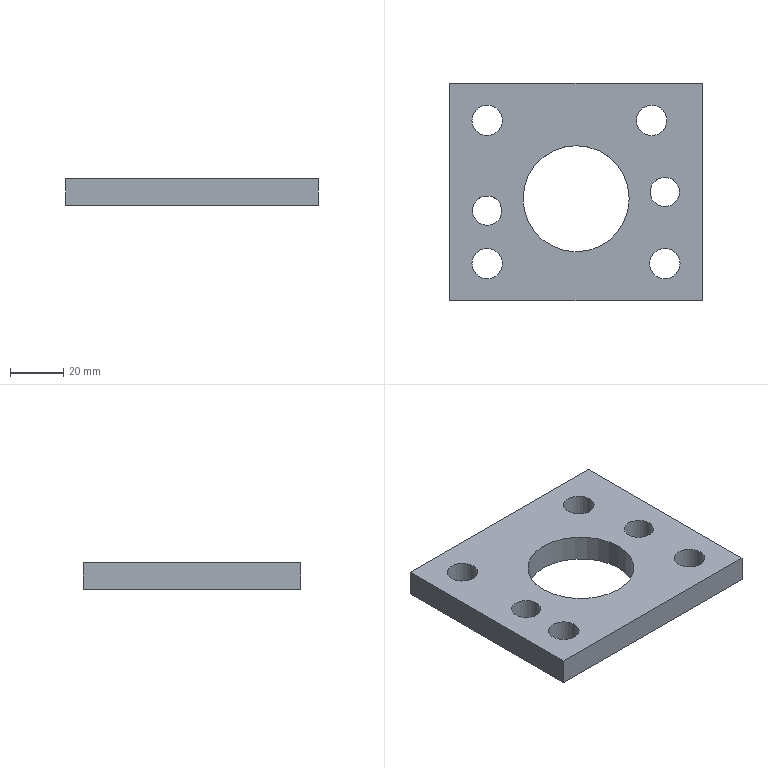Part | STEP file | lll_id4254_x_t | 1 solid | 13 faces | box 95 x 82 x 10 mm | volume 59272 mm3 | cylinder 7 | plane 6 | commonest cylinder face diameters 11.509 x4 11 x2 40 x1
STEP:
#1=CARTESIAN_POINT('',(3157.935,-12.75,-35.));
#2=VERTEX_POINT('',#1);
#3=CARTESIAN_POINT('',(3157.935,-12.75,-45.));
#4=VERTEX_POINT('',#3);
#5=CARTESIAN_POINT('',(3157.935,-12.75,-35.));
#6=DIRECTION('',(0.,0.,-1.));
#7=VECTOR('',#6,1.);
#8=LINE('',#5,#7);
#9=EDGE_CURVE('',#2,#4,#8,.T.);
#10=ORIENTED_EDGE('',*,*,#9,.F.);
#11=CARTESIAN_POINT('',(3252.935,-12.75,-35.));
#12=VERTEX_POINT('',#11);
#13=CARTESIAN_POINT('',(3266.435,-12.75,-35.));
#14=DIRECTION('',(1.,0.,0.));
#15=VECTOR('',#14,1.);
#16=LINE('',#13,#15);
#17=EDGE_CURVE('',#2,#12,#16,.T.);
#18=ORIENTED_EDGE('',*,*,#17,.T.);
#19=CARTESIAN_POINT('',(3252.935,-12.75,-45.));
#20=VERTEX_POINT('',#19);
#21=CARTESIAN_POINT('',(3252.935,-12.75,-35.));
#22=DIRECTION('',(0.,0.,-1.));
#23=VECTOR('',#22,1.);
#24=LINE('',#21,#23);
#25=EDGE_CURVE('',#12,#20,#24,.T.);
#26=ORIENTED_EDGE('',*,*,#25,.T.);
#27=CARTESIAN_POINT('',(3266.435,-12.75,-45.));
#28=DIRECTION('',(1.,0.,0.));
#29=VECTOR('',#28,1.);
#30=LINE('',#27,#29);
#31=EDGE_CURVE('',#4,#20,#30,.T.);
#32=ORIENTED_EDGE('',*,*,#31,.F.);
#33=EDGE_LOOP('',(#10,#18,#26,#32));
#34=FACE_OUTER_BOUND('',#33,.T.);
#35=CARTESIAN_POINT('',(3266.435,-12.75,-35.));
#36=DIRECTION('',(0.,1.,0.));
#37=DIRECTION('',(1.,0.,0.));
#38=AXIS2_PLACEMENT_3D('',#35,#36,#37);
#39=PLANE('',#38);
#40=ADVANCED_FACE('',(#34),#39,.T.);
#41=ORIENTED_EDGE('',*,*,#25,.F.);
#42=CARTESIAN_POINT('',(3252.935,-94.75,-35.));
#43=VERTEX_POINT('',#42);
#44=CARTESIAN_POINT('',(3252.935,-215.25,-35.));
#45=DIRECTION('',(0.,-1.,0.));
#46=VECTOR('',#45,1.);
#47=LINE('',#44,#46);
#48=EDGE_CURVE('',#12,#43,#47,.T.);
#49=ORIENTED_EDGE('',*,*,#48,.T.);
#50=CARTESIAN_POINT('',(3252.935,-94.75,-45.));
#51=VERTEX_POINT('',#50);
#52=CARTESIAN_POINT('',(3252.935,-94.75,-35.));
#53=DIRECTION('',(0.,0.,-1.));
#54=VECTOR('',#53,1.);
#55=LINE('',#52,#54);
#56=EDGE_CURVE('',#43,#51,#55,.T.);
#57=ORIENTED_EDGE('',*,*,#56,.T.);
#58=CARTESIAN_POINT('',(3252.935,-215.25,-45.));
#59=DIRECTION('',(0.,-1.,0.));
#60=VECTOR('',#59,1.);
#61=LINE('',#58,#60);
#62=EDGE_CURVE('',#20,#51,#61,.T.);
#63=ORIENTED_EDGE('',*,*,#62,.F.);
#64=EDGE_LOOP('',(#41,#49,#57,#63));
#65=FACE_OUTER_BOUND('',#64,.T.);
#66=CARTESIAN_POINT('',(3252.935,-215.25,-35.));
#67=DIRECTION('',(1.,0.,0.));
#68=DIRECTION('',(0.,-1.,0.));
#69=AXIS2_PLACEMENT_3D('',#66,#67,#68);
#70=PLANE('',#69);
#71=ADVANCED_FACE('',(#65),#70,.T.);
#72=ORIENTED_EDGE('',*,*,#56,.F.);
#73=CARTESIAN_POINT('',(3157.935,-94.75,-35.));
#74=VERTEX_POINT('',#73);
#75=CARTESIAN_POINT('',(3266.435,-94.75,-35.));
#76=DIRECTION('',(-1.,0.,0.));
#77=VECTOR('',#76,1.);
#78=LINE('',#75,#77);
#79=EDGE_CURVE('',#43,#74,#78,.T.);
#80=ORIENTED_EDGE('',*,*,#79,.T.);
#81=CARTESIAN_POINT('',(3157.935,-94.75,-45.));
#82=VERTEX_POINT('',#81);
#83=CARTESIAN_POINT('',(3157.935,-94.75,-35.));
#84=DIRECTION('',(0.,0.,-1.));
#85=VECTOR('',#84,1.);
#86=LINE('',#83,#85);
#87=EDGE_CURVE('',#74,#82,#86,.T.);
#88=ORIENTED_EDGE('',*,*,#87,.T.);
#89=CARTESIAN_POINT('',(3266.435,-94.75,-45.));
#90=DIRECTION('',(-1.,0.,0.));
#91=VECTOR('',#90,1.);
#92=LINE('',#89,#91);
#93=EDGE_CURVE('',#51,#82,#92,.T.);
#94=ORIENTED_EDGE('',*,*,#93,.F.);
#95=EDGE_LOOP('',(#72,#80,#88,#94));
#96=FACE_OUTER_BOUND('',#95,.T.);
#97=CARTESIAN_POINT('',(3266.435,-94.75,-35.));
#98=DIRECTION('',(0.,-1.,0.));
#99=DIRECTION('',(-1.,0.,0.));
#100=AXIS2_PLACEMENT_3D('',#97,#98,#99);
#101=PLANE('',#100);
#102=ADVANCED_FACE('',(#96),#101,.T.);
#103=CARTESIAN_POINT('',(3233.181,-80.75,-45.));
#104=VERTEX_POINT('',#103);
#105=CARTESIAN_POINT('',(3238.935,-80.75,-45.));
#106=DIRECTION('',(0.,0.,-1.));
#107=DIRECTION('',(-1.,0.,0.));
#108=AXIS2_PLACEMENT_3D('',#105,#106,#107);
#109=CIRCLE('',#108,5.755);
#110=EDGE_CURVE('',#104,#104,#109,.T.);
#111=ORIENTED_EDGE('',*,*,#110,.T.);
#112=EDGE_LOOP('',(#111));
#113=FACE_BOUND('',#112,.T.);
#114=CARTESIAN_POINT('',(3233.181,-80.75,-35.));
#115=VERTEX_POINT('',#114);
#116=CARTESIAN_POINT('',(3238.935,-80.75,-35.));
#117=DIRECTION('',(0.,0.,-1.));
#118=DIRECTION('',(-1.,0.,0.));
#119=AXIS2_PLACEMENT_3D('',#116,#117,#118);
#120=CIRCLE('',#119,5.755);
#121=EDGE_CURVE('',#115,#115,#120,.T.);
#122=ORIENTED_EDGE('',*,*,#121,.F.);
#123=EDGE_LOOP('',(#122));
#124=FACE_BOUND('',#123,.T.);
#125=CARTESIAN_POINT('',(3238.935,-80.75,-35.));
#126=DIRECTION('',(0.,0.,-1.));
#127=DIRECTION('',(-1.,0.,0.));
#128=AXIS2_PLACEMENT_3D('',#125,#126,#127);
#129=CYLINDRICAL_SURFACE('',#128,5.755);
#130=ADVANCED_FACE('',(#113,#124),#129,.F.);
#131=CARTESIAN_POINT('',(3233.435,-53.75,-45.));
#132=VERTEX_POINT('',#131);
#133=CARTESIAN_POINT('',(3238.935,-53.75,-45.));
#134=DIRECTION('',(0.,0.,-1.));
#135=DIRECTION('',(-1.,0.,0.));
#136=AXIS2_PLACEMENT_3D('',#133,#134,#135);
#137=CIRCLE('',#136,5.5);
#138=EDGE_CURVE('',#132,#132,#137,.T.);
#139=ORIENTED_EDGE('',*,*,#138,.T.);
#140=EDGE_LOOP('',(#139));
#141=FACE_BOUND('',#140,.T.);
#142=CARTESIAN_POINT('',(3233.435,-53.75,-35.));
#143=VERTEX_POINT('',#142);
#144=CARTESIAN_POINT('',(3238.935,-53.75,-35.));
#145=DIRECTION('',(0.,0.,-1.));
#146=DIRECTION('',(-1.,0.,0.));
#147=AXIS2_PLACEMENT_3D('',#144,#145,#146);
#148=CIRCLE('',#147,5.5);
#149=EDGE_CURVE('',#143,#143,#148,.T.);
#150=ORIENTED_EDGE('',*,*,#149,.F.);
#151=EDGE_LOOP('',(#150));
#152=FACE_BOUND('',#151,.T.);
#153=CARTESIAN_POINT('',(3238.935,-53.75,-35.));
#154=DIRECTION('',(0.,0.,-1.));
#155=DIRECTION('',(-1.,0.,0.));
#156=AXIS2_PLACEMENT_3D('',#153,#154,#155);
#157=CYLINDRICAL_SURFACE('',#156,5.5);
#158=ADVANCED_FACE('',(#141,#152),#157,.F.);
#159=CARTESIAN_POINT('',(3228.181,-26.75,-45.));
#160=VERTEX_POINT('',#159);
#161=CARTESIAN_POINT('',(3233.935,-26.75,-45.));
#162=DIRECTION('',(0.,0.,-1.));
#163=DIRECTION('',(-1.,0.,0.));
#164=AXIS2_PLACEMENT_3D('',#161,#162,#163);
#165=CIRCLE('',#164,5.755);
#166=EDGE_CURVE('',#160,#160,#165,.T.);
#167=ORIENTED_EDGE('',*,*,#166,.T.);
#168=EDGE_LOOP('',(#167));
#169=FACE_BOUND('',#168,.T.);
#170=CARTESIAN_POINT('',(3228.181,-26.75,-35.));
#171=VERTEX_POINT('',#170);
#172=CARTESIAN_POINT('',(3233.935,-26.75,-35.));
#173=DIRECTION('',(0.,0.,-1.));
#174=DIRECTION('',(-1.,0.,0.));
#175=AXIS2_PLACEMENT_3D('',#172,#173,#174);
#176=CIRCLE('',#175,5.755);
#177=EDGE_CURVE('',#171,#171,#176,.T.);
#178=ORIENTED_EDGE('',*,*,#177,.F.);
#179=EDGE_LOOP('',(#178));
#180=FACE_BOUND('',#179,.T.);
#181=CARTESIAN_POINT('',(3233.935,-26.75,-35.));
#182=DIRECTION('',(0.,0.,-1.));
#183=DIRECTION('',(-1.,0.,0.));
#184=AXIS2_PLACEMENT_3D('',#181,#182,#183);
#185=CYLINDRICAL_SURFACE('',#184,5.755);
#186=ADVANCED_FACE('',(#169,#180),#185,.F.);
#187=CARTESIAN_POINT('',(3166.435,-60.75,-45.));
#188=VERTEX_POINT('',#187);
#189=CARTESIAN_POINT('',(3171.935,-60.75,-45.));
#190=DIRECTION('',(0.,0.,-1.));
#191=DIRECTION('',(-1.,0.,0.));
#192=AXIS2_PLACEMENT_3D('',#189,#190,#191);
#193=CIRCLE('',#192,5.5);
#194=EDGE_CURVE('',#188,#188,#193,.T.);
#195=ORIENTED_EDGE('',*,*,#194,.T.);
#196=EDGE_LOOP('',(#195));
#197=FACE_BOUND('',#196,.T.);
#198=CARTESIAN_POINT('',(3166.435,-60.75,-35.));
#199=VERTEX_POINT('',#198);
#200=CARTESIAN_POINT('',(3171.935,-60.75,-35.));
#201=DIRECTION('',(0.,0.,-1.));
#202=DIRECTION('',(-1.,0.,0.));
#203=AXIS2_PLACEMENT_3D('',#200,#201,#202);
#204=CIRCLE('',#203,5.5);
#205=EDGE_CURVE('',#199,#199,#204,.T.);
#206=ORIENTED_EDGE('',*,*,#205,.F.);
#207=EDGE_LOOP('',(#206));
#208=FACE_BOUND('',#207,.T.);
#209=CARTESIAN_POINT('',(3171.935,-60.75,-35.));
#210=DIRECTION('',(0.,0.,-1.));
#211=DIRECTION('',(-1.,0.,0.));
#212=AXIS2_PLACEMENT_3D('',#209,#210,#211);
#213=CYLINDRICAL_SURFACE('',#212,5.5);
#214=ADVANCED_FACE('',(#197,#208),#213,.F.);
#215=CARTESIAN_POINT('',(3166.181,-26.75,-45.));
#216=VERTEX_POINT('',#215);
#217=CARTESIAN_POINT('',(3171.935,-26.75,-45.));
#218=DIRECTION('',(0.,0.,-1.));
#219=DIRECTION('',(-1.,0.,0.));
#220=AXIS2_PLACEMENT_3D('',#217,#218,#219);
#221=CIRCLE('',#220,5.755);
#222=EDGE_CURVE('',#216,#216,#221,.T.);
#223=ORIENTED_EDGE('',*,*,#222,.T.);
#224=EDGE_LOOP('',(#223));
#225=FACE_BOUND('',#224,.T.);
#226=CARTESIAN_POINT('',(3166.181,-26.75,-35.));
#227=VERTEX_POINT('',#226);
#228=CARTESIAN_POINT('',(3171.935,-26.75,-35.));
#229=DIRECTION('',(0.,0.,-1.));
#230=DIRECTION('',(-1.,0.,0.));
#231=AXIS2_PLACEMENT_3D('',#228,#229,#230);
#232=CIRCLE('',#231,5.755);
#233=EDGE_CURVE('',#227,#227,#232,.T.);
#234=ORIENTED_EDGE('',*,*,#233,.F.);
#235=EDGE_LOOP('',(#234));
#236=FACE_BOUND('',#235,.T.);
#237=CARTESIAN_POINT('',(3171.935,-26.75,-35.));
#238=DIRECTION('',(0.,0.,-1.));
#239=DIRECTION('',(-1.,0.,0.));
#240=AXIS2_PLACEMENT_3D('',#237,#238,#239);
#241=CYLINDRICAL_SURFACE('',#240,5.755);
#242=ADVANCED_FACE('',(#225,#236),#241,.F.);
#243=CARTESIAN_POINT('',(3166.181,-80.75,-45.));
#244=VERTEX_POINT('',#243);
#245=CARTESIAN_POINT('',(3171.935,-80.75,-45.));
#246=DIRECTION('',(0.,0.,-1.));
#247=DIRECTION('',(-1.,0.,0.));
#248=AXIS2_PLACEMENT_3D('',#245,#246,#247);
#249=CIRCLE('',#248,5.755);
#250=EDGE_CURVE('',#244,#244,#249,.T.);
#251=ORIENTED_EDGE('',*,*,#250,.T.);
#252=EDGE_LOOP('',(#251));
#253=FACE_BOUND('',#252,.T.);
#254=CARTESIAN_POINT('',(3166.181,-80.75,-35.));
#255=VERTEX_POINT('',#254);
#256=CARTESIAN_POINT('',(3171.935,-80.75,-35.));
#257=DIRECTION('',(0.,0.,-1.));
#258=DIRECTION('',(-1.,0.,0.));
#259=AXIS2_PLACEMENT_3D('',#256,#257,#258);
#260=CIRCLE('',#259,5.755);
#261=EDGE_CURVE('',#255,#255,#260,.T.);
#262=ORIENTED_EDGE('',*,*,#261,.F.);
#263=EDGE_LOOP('',(#262));
#264=FACE_BOUND('',#263,.T.);
#265=CARTESIAN_POINT('',(3171.935,-80.75,-35.));
#266=DIRECTION('',(0.,0.,-1.));
#267=DIRECTION('',(-1.,0.,0.));
#268=AXIS2_PLACEMENT_3D('',#265,#266,#267);
#269=CYLINDRICAL_SURFACE('',#268,5.755);
#270=ADVANCED_FACE('',(#253,#264),#269,.F.);
#271=CARTESIAN_POINT('',(3157.935,-215.25,-35.));
#272=DIRECTION('',(0.,1.,0.));
#273=VECTOR('',#272,1.);
#274=LINE('',#271,#273);
#275=EDGE_CURVE('',#74,#2,#274,.T.);
#276=ORIENTED_EDGE('',*,*,#275,.T.);
#277=ORIENTED_EDGE('',*,*,#9,.T.);
#278=CARTESIAN_POINT('',(3157.935,-215.25,-45.));
#279=DIRECTION('',(0.,1.,0.));
#280=VECTOR('',#279,1.);
#281=LINE('',#278,#280);
#282=EDGE_CURVE('',#82,#4,#281,.T.);
#283=ORIENTED_EDGE('',*,*,#282,.F.);
#284=ORIENTED_EDGE('',*,*,#87,.F.);
#285=EDGE_LOOP('',(#276,#277,#283,#284));
#286=FACE_OUTER_BOUND('',#285,.T.);
#287=CARTESIAN_POINT('',(3157.935,-215.25,-35.));
#288=DIRECTION('',(-1.,0.,0.));
#289=DIRECTION('',(0.,1.,0.));
#290=AXIS2_PLACEMENT_3D('',#287,#288,#289);
#291=PLANE('',#290);
#292=ADVANCED_FACE('',(#286),#291,.T.);
#293=CARTESIAN_POINT('',(3185.477,-56.288,-45.));
#294=VERTEX_POINT('',#293);
#295=CARTESIAN_POINT('',(3205.477,-56.288,-45.));
#296=DIRECTION('',(0.,0.,-1.));
#297=DIRECTION('',(-1.,0.,0.));
#298=AXIS2_PLACEMENT_3D('',#295,#296,#297);
#299=CIRCLE('',#298,20.);
#300=EDGE_CURVE('',#294,#294,#299,.T.);
#301=ORIENTED_EDGE('',*,*,#300,.T.);
#302=EDGE_LOOP('',(#301));
#303=FACE_BOUND('',#302,.T.);
#304=CARTESIAN_POINT('',(3185.477,-56.288,-35.));
#305=VERTEX_POINT('',#304);
#306=CARTESIAN_POINT('',(3205.477,-56.288,-35.));
#307=DIRECTION('',(0.,0.,-1.));
#308=DIRECTION('',(-1.,0.,0.));
#309=AXIS2_PLACEMENT_3D('',#306,#307,#308);
#310=CIRCLE('',#309,20.);
#311=EDGE_CURVE('',#305,#305,#310,.T.);
#312=ORIENTED_EDGE('',*,*,#311,.F.);
#313=EDGE_LOOP('',(#312));
#314=FACE_BOUND('',#313,.T.);
#315=CARTESIAN_POINT('',(3205.477,-56.288,-35.));
#316=DIRECTION('',(0.,0.,1.));
#317=DIRECTION('',(1.,0.,0.));
#318=AXIS2_PLACEMENT_3D('',#315,#316,#317);
#319=CYLINDRICAL_SURFACE('',#318,20.);
#320=ADVANCED_FACE('',(#303,#314),#319,.F.);
#321=ORIENTED_EDGE('',*,*,#110,.F.);
#322=EDGE_LOOP('',(#321));
#323=FACE_BOUND('',#322,.T.);
#324=ORIENTED_EDGE('',*,*,#138,.F.);
#325=EDGE_LOOP('',(#324));
#326=FACE_BOUND('',#325,.T.);
#327=ORIENTED_EDGE('',*,*,#166,.F.);
#328=EDGE_LOOP('',(#327));
#329=FACE_BOUND('',#328,.T.);
#330=ORIENTED_EDGE('',*,*,#194,.F.);
#331=EDGE_LOOP('',(#330));
#332=FACE_BOUND('',#331,.T.);
#333=ORIENTED_EDGE('',*,*,#222,.F.);
#334=EDGE_LOOP('',(#333));
#335=FACE_BOUND('',#334,.T.);
#336=ORIENTED_EDGE('',*,*,#250,.F.);
#337=EDGE_LOOP('',(#336));
#338=FACE_BOUND('',#337,.T.);
#339=ORIENTED_EDGE('',*,*,#93,.T.);
#340=ORIENTED_EDGE('',*,*,#282,.T.);
#341=ORIENTED_EDGE('',*,*,#31,.T.);
#342=ORIENTED_EDGE('',*,*,#62,.T.);
#343=EDGE_LOOP('',(#339,#340,#341,#342));
#344=FACE_BOUND('',#343,.T.);
#345=ORIENTED_EDGE('',*,*,#300,.F.);
#346=EDGE_LOOP('',(#345));
#347=FACE_BOUND('',#346,.T.);
#348=CARTESIAN_POINT('',(3266.435,-215.25,-45.));
#349=DIRECTION('',(0.,0.,-1.));
#350=DIRECTION('',(1.,0.,0.));
#351=AXIS2_PLACEMENT_3D('',#348,#349,#350);
#352=PLANE('',#351);
#353=ADVANCED_FACE('',(#323,#326,#329,#332,#335,#338,#344,#347),#352,.T.);
#354=ORIENTED_EDGE('',*,*,#121,.T.);
#355=EDGE_LOOP('',(#354));
#356=FACE_BOUND('',#355,.T.);
#357=ORIENTED_EDGE('',*,*,#149,.T.);
#358=EDGE_LOOP('',(#357));
#359=FACE_BOUND('',#358,.T.);
#360=ORIENTED_EDGE('',*,*,#177,.T.);
#361=EDGE_LOOP('',(#360));
#362=FACE_BOUND('',#361,.T.);
#363=ORIENTED_EDGE('',*,*,#205,.T.);
#364=EDGE_LOOP('',(#363));
#365=FACE_BOUND('',#364,.T.);
#366=ORIENTED_EDGE('',*,*,#233,.T.);
#367=EDGE_LOOP('',(#366));
#368=FACE_BOUND('',#367,.T.);
#369=ORIENTED_EDGE('',*,*,#261,.T.);
#370=EDGE_LOOP('',(#369));
#371=FACE_BOUND('',#370,.T.);
#372=ORIENTED_EDGE('',*,*,#79,.F.);
#373=ORIENTED_EDGE('',*,*,#48,.F.);
#374=ORIENTED_EDGE('',*,*,#17,.F.);
#375=ORIENTED_EDGE('',*,*,#275,.F.);
#376=EDGE_LOOP('',(#372,#373,#374,#375));
#377=FACE_BOUND('',#376,.T.);
#378=ORIENTED_EDGE('',*,*,#311,.T.);
#379=EDGE_LOOP('',(#378));
#380=FACE_BOUND('',#379,.T.);
#381=CARTESIAN_POINT('',(3266.435,-215.25,-35.));
#382=DIRECTION('',(0.,0.,-1.));
#383=DIRECTION('',(1.,0.,0.));
#384=AXIS2_PLACEMENT_3D('',#381,#382,#383);
#385=PLANE('',#384);
#386=ADVANCED_FACE('',(#356,#359,#362,#365,#368,#371,#377,#380),#385,.F.);
#387=CLOSED_SHELL('',(#40,#71,#102,#130,#158,#186,#214,#242,#270,#292,#320,#353,#386));
#388=MANIFOLD_SOLID_BREP('',#387);
#389=(LENGTH_UNIT()NAMED_UNIT(*)SI_UNIT(.MILLI.,.METRE.));
#390=UNCERTAINTY_MEASURE_WITH_UNIT(LENGTH_MEASURE(0.00002),#389,'','');
#391=(NAMED_UNIT(*)PLANE_ANGLE_UNIT()SI_UNIT($,.RADIAN.));
#392=PLANE_ANGLE_MEASURE_WITH_UNIT(PLANE_ANGLE_MEASURE(0.01745),#391);
#393=DIMENSIONAL_EXPONENTS(0.,0.,0.,0.,0.,0.,0.);
#394=(CONVERSION_BASED_UNIT('DEGREE',#392)NAMED_UNIT(#393)PLANE_ANGLE_UNIT());
#395=(NAMED_UNIT(*)SI_UNIT($,.STERADIAN.)SOLID_ANGLE_UNIT());
#396=(GEOMETRIC_REPRESENTATION_CONTEXT(3)GLOBAL_UNCERTAINTY_ASSIGNED_CONTEXT((#390))GLOBAL_UNIT_ASSIGNED_CONTEXT((#389,#394,#395))REPRESENTATION_CONTEXT('',''));
#397=ADVANCED_BREP_SHAPE_REPRESENTATION('',(#388),#396);